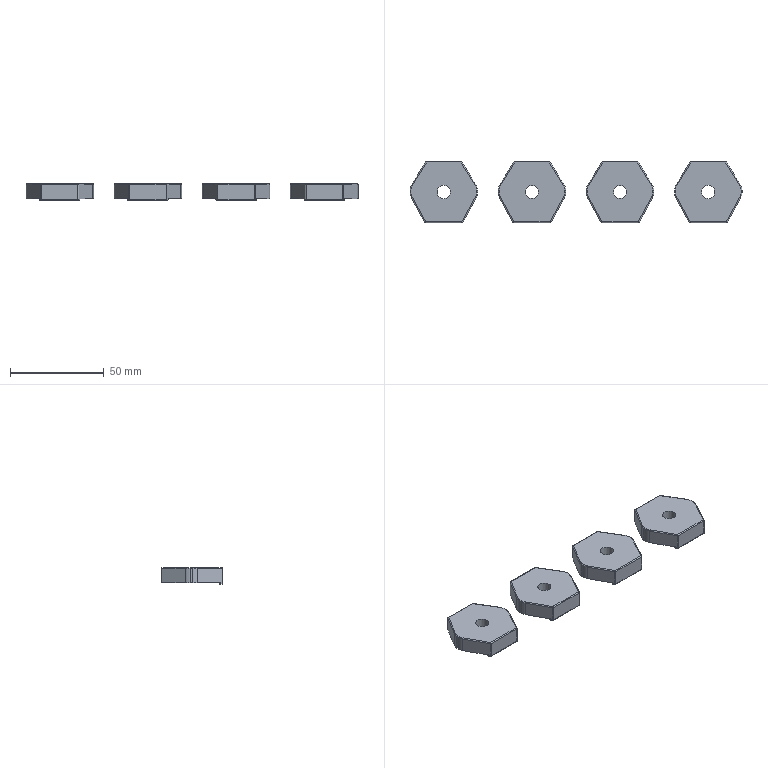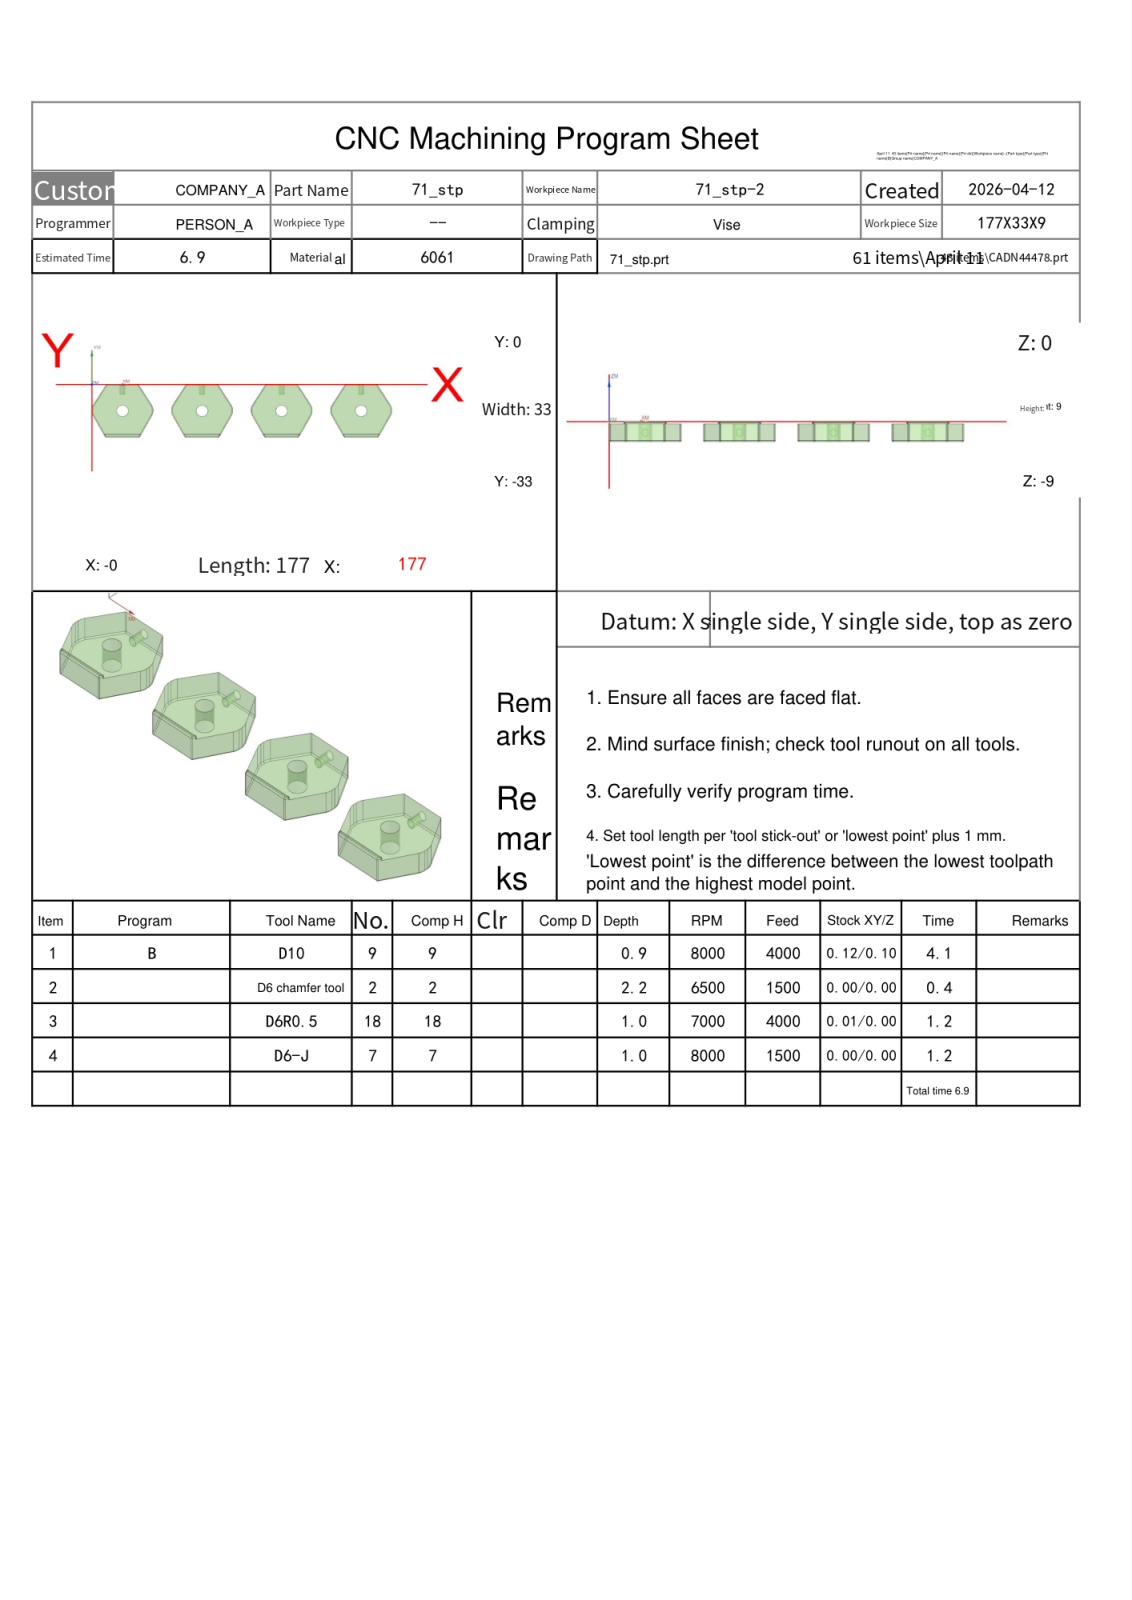NC program | NX | posted by the shop | part box 177 x 33 x 9 mm
Lines 2353 to 3592 of 12693:
N3 T18 M06
(D6R0.5  D=6. R=0.5 H=18 ce=0.01 di=0.00)
G00 G90 G54 X149.909 Y-28.832 M03 S7000
G43 H18 Z50.
M08
Z1.5
G01 X169.408 Z.478 F4000.
X169.836 Y-28.894 Z.455
X170.249 Y-29.023 Z.433
X170.635 Y-29.218 Z.41
X170.985 Y-29.472 Z.387
X171.29 Y-29.78 Z.365
X171.54 Y-30.133 Z.342
X171.731 Y-30.521 Z.319
X171.856 Y-30.935 Z.297
X171.913 Y-31.364 Z.274
X171.9 Y-31.797 Z.251
X171.817 Y-32.221 Z.229
X171.667 Y-32.627 Z.206
X170.97 Y-33.915 Z.129
X170.718 Y-34.255 Z.107
X170.415 Y-34.551 Z.085
X170.07 Y-34.796 Z.063
X169.69 Y-34.983 Z.04
X169.285 Y-35.108 Z.018
X168.866 Y-35.168 Z-.004
X168.702 Z-.012
X149.298
G02 X146.952 Y-33.771 I0.0 J2.668
G01 X146.411 Y-32.771
G02 X146.088 Y-31.5 I2.345 J1.271
X148.756 Y-28.832 I2.668 J0.0
G01 X169.244
G02 X171.912 Y-31.5 I0.0 J-2.668
X171.589 Y-32.771 I-2.668 J0.0
G01 X171.048 Y-33.771
G02 X168.702 Y-35.168 I-2.345 J1.271
G01 X166.277 Y-35.173 Z-.013
X163.851 Y-35.178 Z-.014
X161.426 Y-35.183 Z-.015
X159. Y-35.188 Z-.016
X156.574 Y-35.193 Z-.017
X154.149 Y-35.197 Z-.018
X151.723 Y-35.203 Z-.019
X149.298 Y-35.207 Z-.02
X149.217 Y-35.206
X149.136 Y-35.202
X149.056 Y-35.197
X148.975 Y-35.188
X148.895 Y-35.178
X148.816 Y-35.165
X148.736 Y-35.149
X148.657 Y-35.131
X148.579 Y-35.111
X148.502 Y-35.089
X148.425 Y-35.064
X148.349 Y-35.037
X148.273 Y-35.008
X148.199 Y-34.976
X148.125 Y-34.942
X148.053 Y-34.906
X147.981 Y-34.868
X147.911 Y-34.828
X147.842 Y-34.786
X147.775 Y-34.741
X147.644 Y-34.647
X147.518 Y-34.544
X147.399 Y-34.435
X147.287 Y-34.318 Z-.021
X147.182 Y-34.196
X147.084 Y-34.067
X146.995 Y-33.932
X146.913 Y-33.792
X146.641 Y-33.293
X146.369 Y-32.793
X146.331 Y-32.72
X146.295 Y-32.646
X146.261 Y-32.571
X146.23 Y-32.494
X146.2 Y-32.417
X146.174 Y-32.339
X146.149 Y-32.26
X146.127 Y-32.181
X146.107 Y-32.1
X146.09 Y-32.02
X146.075 Y-31.938 Z-.022
X146.063 Y-31.857
X146.053 Y-31.775
X146.046 Y-31.693
X146.041 Y-31.61
X146.039 Y-31.528
Y-31.445
X146.042 Y-31.362
X146.047 Y-31.28
X146.055 Y-31.198
X146.066 Y-31.116
X146.078 Y-31.034
X146.094 Y-30.953
X146.111 Y-30.872
X146.132 Y-30.792
X146.154 Y-30.713
X146.179 Y-30.634
X146.206 Y-30.556
X146.236 Y-30.479
X146.268 Y-30.402
X146.303 Y-30.327
X146.339 Y-30.253
X146.378 Y-30.18
X146.419 Y-30.109
X146.463 Y-30.038
X146.508 Y-29.969
X146.555 Y-29.901
X146.605 Y-29.835
X146.656 Y-29.77
X146.71 Y-29.707
X146.765 Y-29.646
X146.822 Y-29.586
X146.881 Y-29.528
X146.942 Y-29.472 Z-.023
X147.004 Y-29.418
X147.069 Y-29.365
X147.134 Y-29.315
X147.201 Y-29.266
X147.27 Y-29.22
X147.34 Y-29.176
X147.411 Y-29.134
X147.483 Y-29.094
X147.557 Y-29.056
X147.632 Y-29.021
X147.708 Y-28.987
X147.785 Y-28.957
X147.862 Y-28.928
X147.941 Y-28.902
X148.02 Y-28.878
X148.1 Y-28.857
X148.181 Y-28.838
X148.262 Y-28.822
X148.343 Y-28.808
X148.426 Y-28.797
X148.508 Y-28.787
X148.59 Y-28.781
X148.673 Y-28.777
X148.756 Y-28.776
X151.317 Y-28.772 Z-.024
X153.878 Y-28.768 Z-.025
X156.439 Y-28.763 Z-.026
X159. Y-28.76 Z-.027
X161.561 Y-28.755 Z-.028
X164.122 Y-28.752 Z-.029
X166.683 Y-28.747 Z-.03
X169.244 Y-28.744 Z-.031
X169.328 Y-28.745
X169.412 Y-28.748
X169.495 Y-28.755
X169.579 Y-28.763
X169.662 Y-28.775
X169.744 Y-28.789
X169.826 Y-28.805
X169.908 Y-28.824
X169.989 Y-28.845
X170.07 Y-28.869
X170.149 Y-28.895
X170.228 Y-28.924
X170.306 Y-28.955
X170.383 Y-28.988
X170.459 Y-29.024
X170.534 Y-29.062
X170.607 Y-29.102
X170.679 Y-29.144
X170.751 Y-29.189
X170.82 Y-29.236
X170.888 Y-29.285 Z-.032
X170.955 Y-29.335
X171.02 Y-29.388
X171.083 Y-29.443
X171.145 Y-29.5
X171.205 Y-29.559
X171.263 Y-29.619
X171.32 Y-29.681
X171.374 Y-29.745
X171.427 Y-29.811
X171.477 Y-29.878
X171.525 Y-29.946
X171.572 Y-30.016
X171.616 Y-30.088
X171.658 Y-30.16
X171.697 Y-30.234
X171.735 Y-30.309
X171.77 Y-30.386
X171.803 Y-30.463
X171.833 Y-30.541
X171.862 Y-30.62
X171.887 Y-30.7
X171.91 Y-30.781
X171.931 Y-30.862
X171.949 Y-30.944
X171.965 Y-31.027
X171.978 Y-31.109
X171.989 Y-31.193
X171.997 Y-31.276
X172.003 Y-31.36
X172.006 Y-31.444
Y-31.528
X172.005 Y-31.612 Z-.033
X172. Y-31.696
X171.993 Y-31.78
X171.983 Y-31.863
X171.971 Y-31.946
X171.956 Y-32.029
X171.939 Y-32.111
X171.919 Y-32.193
X171.897 Y-32.274
X171.872 Y-32.354
X171.846 Y-32.434
X171.816 Y-32.512
X171.784 Y-32.59
X171.75 Y-32.667
X171.714 Y-32.743
X171.674 Y-32.817
X171.404 Y-33.317
X171.134 Y-33.818
X171.094 Y-33.89
X171.051 Y-33.961
X171.007 Y-34.03
X170.96 Y-34.098 Z-.034
X170.912 Y-34.165
X170.861 Y-34.23
X170.809 Y-34.294
X170.754 Y-34.356
X170.698 Y-34.417
X170.64 Y-34.475
X170.58 Y-34.532
X170.519 Y-34.587
X170.456 Y-34.641
X170.391 Y-34.692
X170.325 Y-34.742
X170.258 Y-34.789
X170.189 Y-34.835
X170.118 Y-34.878
X170.047 Y-34.92
X169.974 Y-34.958
X169.9 Y-34.996
X169.825 Y-35.03
X169.75 Y-35.063
X169.672 Y-35.093
X169.595 Y-35.121
X169.516 Y-35.147
X169.437 Y-35.17
X169.357 Y-35.19
X169.276 Y-35.209
X169.195 Y-35.225
X169.114 Y-35.239
X169.032 Y-35.25
X168.867 Y-35.265
X168.702 Y-35.27 Z-.035
X166.277 Y-35.275 Z-.036
X163.851 Y-35.28 Z-.037
X161.426 Y-35.284 Z-.038
X159. Y-35.288 Z-.04
X156.574 Y-35.293 Z-.041
X154.149 Y-35.297 Z-.042
X151.723 Y-35.301 Z-.043
X149.298 Y-35.305 Z-.045
X149.214
X149.13 Y-35.301
X149.047 Y-35.295
X148.964 Y-35.286
X148.881 Y-35.275
X148.798 Y-35.261
X148.716 Y-35.246
X148.634 Y-35.227
X148.553 Y-35.206
X148.473 Y-35.183
X148.393 Y-35.157
X148.314 Y-35.129
X148.236 Y-35.099
X148.159 Y-35.066
X148.083 Y-35.031
X148.008 Y-34.994
X147.934 Y-34.955 Z-.046
X147.861 Y-34.913
X147.789 Y-34.869
X147.72 Y-34.823
X147.651 Y-34.775
X147.584 Y-34.725
X147.518 Y-34.673
X147.454 Y-34.619
X147.391 Y-34.563
X147.331 Y-34.505
X147.271 Y-34.446
X147.214 Y-34.385
X147.159 Y-34.322
X147.105 Y-34.257
X147.053 Y-34.191
X147.004 Y-34.123
X146.956 Y-34.054
X146.911 Y-33.984
X146.868 Y-33.912
X146.827 Y-33.839
X146.555 Y-33.339 Z-.047
X146.283 Y-32.84
X146.21 Y-32.696
X146.145 Y-32.548
X146.089 Y-32.396
X146.042 Y-32.242
X146.004 Y-32.085
X145.974 Y-31.926
X145.954 Y-31.766 Z-.048
X145.943 Y-31.605
X145.942 Y-31.443
X145.949 Y-31.281
X145.966 Y-31.121
X145.992 Y-30.961
X146.027 Y-30.803
X146.072 Y-30.648
X146.125 Y-30.495
X146.186 Y-30.346
X146.257 Y-30.2
X146.335 Y-30.058 Z-.049
X146.422 Y-29.922
X146.516 Y-29.79
X146.618 Y-29.664
X146.726 Y-29.544
X146.842 Y-29.431
X146.963 Y-29.324
X147.091 Y-29.225
X147.224 Y-29.133
X147.363 Y-29.049
X147.505 Y-28.972
X147.652 Y-28.905
X147.803 Y-28.845 Z-.05
X147.957 Y-28.795
X148.114 Y-28.753
X148.272 Y-28.72
X148.433 Y-28.697
X148.594 Y-28.683
X148.756 Y-28.678
X151.317 Y-28.674 Z-.051
X153.878 Y-28.67 Z-.053
X156.439 Y-28.666 Z-.054
X159. Y-28.662 Z-.055
X161.561 Y-28.658 Z-.057
X164.122 Y-28.654 Z-.058
X166.683 Y-28.65 Z-.06
X169.244 Y-28.647 Z-.061
X169.408 Y-28.651
X169.571 Y-28.665
X169.733 Y-28.688
X169.894 Y-28.721
X170.053 Y-28.762
X170.208 Y-28.813
X170.361 Y-28.873
X170.51 Y-28.941 Z-.062
X170.655 Y-29.018
X170.796 Y-29.102
X170.931 Y-29.195
X171.06 Y-29.295
X171.184 Y-29.403
X171.301 Y-29.518
X171.412 Y-29.639
X171.515 Y-29.766
X171.611 Y-29.9
X171.699 Y-30.038
X171.779 Y-30.181 Z-.063
X171.851 Y-30.329
X171.914 Y-30.48
X171.969 Y-30.635
X172.014 Y-30.793
X172.05 Y-30.953
X172.077 Y-31.115
X172.095 Y-31.278
X172.103 Y-31.442
X172.102 Y-31.606
X172.091 Y-31.77
X172.071 Y-31.933
X172.042 Y-32.095 Z-.064
X172.004 Y-32.254
X171.956 Y-32.412
X171.899 Y-32.566
X171.834 Y-32.717
X171.76 Y-32.863
X171.49 Y-33.364
X171.22 Y-33.864 Z-.065
X171.178 Y-33.939
X171.134 Y-34.012
X171.088 Y-34.084
X171.04 Y-34.154
X170.99 Y-34.224
X170.937 Y-34.291
X170.883 Y-34.357
X170.826 Y-34.421
X170.768 Y-34.484
X170.708 Y-34.545
X170.647 Y-34.604
X170.583 Y-34.661
X170.518 Y-34.716
X170.451 Y-34.769
X170.382 Y-34.821
X170.312 Y-34.87
X170.241 Y-34.917
X170.168 Y-34.962
X170.094 Y-35.005
X170.019 Y-35.045 Z-.066
X169.943 Y-35.084
X169.865 Y-35.119
X169.786 Y-35.153
X169.707 Y-35.184
X169.626 Y-35.213
X169.545 Y-35.24
X169.463 Y-35.264
X169.38 Y-35.285
X169.297 Y-35.305
X169.213 Y-35.321
X169.128 Y-35.335
X169.044 Y-35.347
X168.959 Y-35.356
X168.873 Y-35.362
X168.788 Y-35.366
X168.702 Y-35.368
X166.277 Y-35.372 Z-.068
X163.851 Y-35.376 Z-.07
X161.426 Y-35.38 Z-.071
X159. Y-35.384 Z-.073
X156.574 Y-35.388 Z-.074
X154.149 Y-35.392 Z-.076
X151.723 Y-35.396 Z-.078
X149.298 Y-35.4 Z-.079
X149.142 Y-35.396
X148.987 Y-35.384 Z-.08
X148.832 Y-35.363
X148.679 Y-35.334
X148.528 Y-35.297
X148.379 Y-35.252
X148.232 Y-35.199
X148.089 Y-35.138
X147.949 Y-35.07
X147.813 Y-34.994
X147.681 Y-34.911 Z-.081
X147.554 Y-34.821
X147.431 Y-34.724
X147.314 Y-34.621
X147.203 Y-34.511
X147.098 Y-34.396
X146.999 Y-34.275
X146.907 Y-34.15
X146.822 Y-34.019
X146.744 Y-33.884
X146.472 Y-33.384 Z-.082
X146.2 Y-32.885
X146.125 Y-32.736
X146.058 Y-32.583
X146. Y-32.426 Z-.083
X145.951 Y-32.267
X145.911 Y-32.105
X145.881 Y-31.94
X145.86 Y-31.775
X145.849 Y-31.608
X145.847 Y-31.441
X145.855 Y-31.274
X145.873 Y-31.108
X145.9 Y-30.943 Z-.084
X145.936 Y-30.78
X145.982 Y-30.619
X146.037 Y-30.461
X146.1 Y-30.307
X146.173 Y-30.156
X146.254 Y-30.01
X146.344 Y-29.869
X146.441 Y-29.733 Z-.085
X146.546 Y-29.603
X146.658 Y-29.479
X146.778 Y-29.362
X146.903 Y-29.251
X147.036 Y-29.149
X147.173 Y-29.054
X147.316 Y-28.967
X147.464 Y-28.888
X147.616 Y-28.818 Z-.086
X147.771 Y-28.756
X147.93 Y-28.704
X148.092 Y-28.661
X148.256 Y-28.628
X148.422 Y-28.603
X148.589 Y-28.589
X148.756 Y-28.584
X151.317 Y-28.58 Z-.088
X153.878 Y-28.576 Z-.09
X156.439 Y-28.573 Z-.092
X159. Y-28.569 Z-.093
X161.561 Y-28.565 Z-.095
X164.122 Y-28.561 Z-.097
X166.683 Y-28.558 Z-.098
X169.244 Y-28.554 Z-.1
X169.413 Y-28.559
X169.582 Y-28.573
X169.749 Y-28.597 Z-.101
X169.915 Y-28.63
X170.079 Y-28.673
X170.24 Y-28.726
X170.397 Y-28.787
X170.551 Y-28.858
X170.701 Y-28.937
X170.846 Y-29.024
X170.985 Y-29.12
X171.119 Y-29.224 Z-.102
X171.247 Y-29.335
X171.368 Y-29.453
X171.482 Y-29.579
X171.589 Y-29.71
X171.688 Y-29.848
X171.779 Y-29.99
X171.862 Y-30.138
X171.936 Y-30.291
X172.001 Y-30.447 Z-.103
X172.057 Y-30.607
X172.104 Y-30.77
X172.141 Y-30.935
X172.169 Y-31.102
X172.188 Y-31.271
X172.196 Y-31.44
X172.195 Y-31.61
X172.184 Y-31.779 Z-.104
X172.163 Y-31.947
X172.133 Y-32.114
X172.093 Y-32.279
X172.044 Y-32.441
X171.986 Y-32.6
X171.918 Y-32.756
X171.842 Y-32.908
X171.571 Y-33.408 Z-.105
X171.301 Y-33.908
X171.222 Y-34.046
X171.136 Y-34.179
X171.042 Y-34.307
X170.942 Y-34.431 Z-.106
X170.835 Y-34.548
X170.722 Y-34.66
X170.604 Y-34.765
X170.479 Y-34.864
X170.35 Y-34.957
X170.216 Y-35.042
X170.077 Y-35.119
X169.935 Y-35.19
X169.789 Y-35.252
X169.639 Y-35.307 Z-.107
X169.487 Y-35.353
X169.333 Y-35.391
X169.177 Y-35.421
X169.02 Y-35.443
X168.861 Y-35.456
X168.702 Y-35.461
X166.277 Y-35.464 Z-.109
X163.851 Y-35.468 Z-.111
X161.426 Y-35.472 Z-.113
X159. Y-35.476 Z-.115
X156.574 Y-35.48 Z-.117
X154.149 Y-35.483 Z-.119
X151.723 Y-35.487 Z-.121
X149.298 Y-35.49 Z-.123
X149.137 Y-35.486
X148.977 Y-35.473
X148.818 Y-35.452
X148.66 Y-35.422 Z-.124
X148.504 Y-35.384
X148.35 Y-35.338
X148.199 Y-35.283
X148.051 Y-35.22
X147.907 Y-35.15
X147.767 Y-35.071
X147.63 Y-34.986 Z-.125
X147.499 Y-34.893
X147.373 Y-34.793
X147.253 Y-34.686
X147.138 Y-34.574
X147.03 Y-34.455
X146.928 Y-34.331
X146.833 Y-34.201
X146.745 Y-34.066 Z-.126
X146.664 Y-33.927
X146.393 Y-33.427
X146.121 Y-32.928 Z-.127
X146.081 Y-32.852
X146.043 Y-32.774
X146.007 Y-32.696
X145.974 Y-32.617
X145.943 Y-32.536
X145.915 Y-32.455
X145.888 Y-32.373
X145.864 Y-32.291
X145.842 Y-32.207
X145.823 Y-32.123
X145.806 Y-32.039
X145.792 Y-31.954
X145.78 Y-31.869 Z-.128
X145.771 Y-31.783
X145.764 Y-31.697
X145.759 Y-31.611
X145.757 Y-31.525
Y-31.439
X145.76 Y-31.353
X145.766 Y-31.267
X145.773 Y-31.181
X145.784 Y-31.096
X145.796 Y-31.011
X145.811 Y-30.926
X145.829 Y-30.842
X145.849 Y-30.758
X145.871 Y-30.675 Z-.129
X145.896 Y-30.592
X145.923 Y-30.51
X145.953 Y-30.429
X145.984 Y-30.349
X146.019 Y-30.27
X146.055 Y-30.192
X146.093 Y-30.115
X146.134 Y-30.039
X146.177 Y-29.964
X146.222 Y-29.891
X146.269 Y-29.819
X146.318 Y-29.748
X146.37 Y-29.679
X146.423 Y-29.611 Z-.13
X146.478 Y-29.544
X146.535 Y-29.48
X146.594 Y-29.417
X146.654 Y-29.355
X146.717 Y-29.296
X146.781 Y-29.238
X146.846 Y-29.182
X146.914 Y-29.128
X146.982 Y-29.076
X147.053 Y-29.026
X147.124 Y-28.978
X147.197 Y-28.932
X147.272 Y-28.889
X147.347 Y-28.847 Z-.131
X147.424 Y-28.807
X147.502 Y-28.77
X147.58 Y-28.735
X147.66 Y-28.703
X147.741 Y-28.672
X147.823 Y-28.644
X147.905 Y-28.618
X147.988 Y-28.595
X148.072 Y-28.574
X148.156 Y-28.555
X148.241 Y-28.539
X148.326 Y-28.526
X148.411 Y-28.514
X148.497 Y-28.506
X148.583 Y-28.499 Z-.132
X148.67 Y-28.495
X148.756 Y-28.494
X151.317 Y-28.491 Z-.134
X153.878 Y-28.487 Z-.136
X156.439 Y-28.484 Z-.138
X159. Y-28.48 Z-.14
X161.561 Y-28.477 Z-.142
X164.122 Y-28.473 Z-.144
X166.683 Y-28.469 Z-.146
X169.244 Y-28.466 Z-.148
X169.331 Y-28.467 Z-.149
X169.418 Y-28.471
X169.505 Y-28.477
X169.592 Y-28.486
X169.678 Y-28.496
X169.764 Y-28.51
X169.85 Y-28.526
X169.935 Y-28.545
X170.02 Y-28.566
X170.104 Y-28.589
X170.187 Y-28.615
X170.269 Y-28.643
X170.351 Y-28.673
X170.432 Y-28.706
X170.512 Y-28.741
X170.59 Y-28.779 Z-.15
X170.668 Y-28.818
X170.744 Y-28.86
X170.82 Y-28.904
X170.894 Y-28.951
X170.966 Y-28.999
X171.037 Y-29.049
X171.107 Y-29.102
X171.175 Y-29.156
X171.242 Y-29.212
X171.307 Y-29.271
X171.37 Y-29.331
X171.431 Y-29.393
X171.491 Y-29.456
X171.549 Y-29.521 Z-.151
X171.605 Y-29.588
X171.659 Y-29.657
X171.711 Y-29.727
X171.761 Y-29.798
X171.809 Y-29.871
X171.855 Y-29.945
X171.898 Y-30.021
X171.94 Y-30.098
X171.979 Y-30.176
X172.016 Y-30.255
X172.051 Y-30.335
X172.083 Y-30.416
X172.113 Y-30.498
X172.141 Y-30.58 Z-.152
X172.166 Y-30.664
X172.189 Y-30.748
X172.21 Y-30.833
X172.228 Y-30.918
X172.243 Y-31.004
X172.256 Y-31.09
X172.267 Y-31.177
X172.275 Y-31.264
X172.281 Y-31.351
X172.284 Y-31.438
Y-31.526
X172.283 Y-31.613
X172.278 Y-31.7
X172.271 Y-31.787 Z-.153
X172.262 Y-31.874
X172.25 Y-31.96
X172.236 Y-32.047
X172.219 Y-32.132
X172.2 Y-32.217
X172.178 Y-32.302
X172.154 Y-32.386
X172.127 Y-32.469
X172.098 Y-32.552
X172.067 Y-32.633
X172.034 Y-32.714
X171.998 Y-32.793
X171.959 Y-32.872
X171.919 Y-32.949 Z-.154
X171.649 Y-33.45
X171.378 Y-33.95
X171.297 Y-34.092 Z-.155
X171.208 Y-34.229
X171.112 Y-34.361
X171.008 Y-34.488
X170.898 Y-34.609
X170.782 Y-34.724
X170.66 Y-34.833
X170.532 Y-34.934 Z-.156
X170.399 Y-35.029
X170.261 Y-35.117
X170.118 Y-35.197
X169.971 Y-35.269
X169.821 Y-35.334
X169.667 Y-35.39
X169.511 Y-35.438
X169.352 Y-35.477 Z-.157
X169.191 Y-35.508
X169.029 Y-35.53
X168.866 Y-35.543
X168.702 Y-35.548
X166.277 Y-35.551 Z-.159
X163.851 Y-35.555 Z-.162
X161.426 Y-35.558 Z-.164
X159. Y-35.562 Z-.166
X156.574 Y-35.566 Z-.169
X154.149 Y-35.569 Z-.171
X151.723 Y-35.573 Z-.173
X149.298 Y-35.575 Z-.176
X149.133 Y-35.571
X148.968 Y-35.558
X148.804 Y-35.536
X148.642 Y-35.506
X148.481 Y-35.466
X148.323 Y-35.418
X148.168 Y-35.362 Z-.177
X148.016 Y-35.298
X147.867 Y-35.225
X147.723 Y-35.144
X147.583 Y-35.056
X147.448 Y-34.961
X147.319 Y-34.858 Z-.178
X147.195 Y-34.749
X147.077 Y-34.633
X146.965 Y-34.51
X146.861 Y-34.382
X146.763 Y-34.249
X146.672 Y-34.111
X146.59 Y-33.967 Z-.179
X146.318 Y-33.468
X146.046 Y-32.968 Z-.18
X145.97 Y-32.819
X145.903 Y-32.665
X145.843 Y-32.509
X145.792 Y-32.349
X145.75 Y-32.186 Z-.181
X145.717 Y-32.022
X145.693 Y-31.856
X145.678 Y-31.689
X145.672 Y-31.521
X145.675 Y-31.354
X145.688 Y-31.186
X145.709 Y-31.02 Z-.182
X145.739 Y-30.855
X145.779 Y-30.692
X145.827 Y-30.531
X145.884 Y-30.373
X145.949 Y-30.218
X146.023 Y-30.068 Z-.183
X146.104 Y-29.921
X146.194 Y-29.779
X146.291 Y-29.642
X146.396 Y-29.511
X146.507 Y-29.385
X146.625 Y-29.266 Z-.184
X146.75 Y-29.153
X146.88 Y-29.047
X147.016 Y-28.949
X147.157 Y-28.858
X147.303 Y-28.775
X147.454 Y-28.699
X147.608 Y-28.633 Z-.185
X147.765 Y-28.574
X147.926 Y-28.524
X148.089 Y-28.483
X148.254 Y-28.451
X148.42 Y-28.428
X148.588 Y-28.415 Z-.186
X148.756 Y-28.41
X151.317 Y-28.406 Z-.188
X153.878 Y-28.403 Z-.191
X156.439 Y-28.4 Z-.193
X159. Y-28.397 Z-.195
X161.561 Y-28.393 Z-.198
X164.122 Y-28.39 Z-.2
X166.683 Y-28.387 Z-.203
X169.244 Y-28.383 Z-.205
X169.414 Y-28.388
X169.583 Y-28.402
X169.751 Y-28.424 Z-.206
X169.917 Y-28.456
X170.082 Y-28.497
X170.244 Y-28.547
X170.403 Y-28.605
X170.559 Y-28.673
X170.711 Y-28.748 Z-.207
X170.858 Y-28.832
X171.001 Y-28.923
X171.139 Y-29.022
X171.271 Y-29.129
X171.397 Y-29.242
X171.517 Y-29.363 Z-.208
X171.63 Y-29.489
X171.736 Y-29.622
X171.834 Y-29.76
X171.925 Y-29.903
X172.008 Y-30.051
X172.083 Y-30.204
X172.15 Y-30.36 Z-.209
X172.207 Y-30.52
X172.257 Y-30.682
X172.297 Y-30.847
X172.328 Y-31.014
X172.35 Y-31.182
X172.363 Y-31.352 Z-.21
X172.367 Y-31.522
X172.361 Y-31.691
X172.346 Y-31.861
X172.322 Y-32.029
X172.289 Y-32.195
X172.247 Y-32.36 Z-.211
X172.196 Y-32.522
X172.136 Y-32.681
X172.068 Y-32.837
X171.991 Y-32.989
X171.721 Y-33.489 Z-.212
X171.45 Y-33.989
X171.367 Y-34.135
X171.275 Y-34.276 Z-.213
X171.176 Y-34.411
X171.071 Y-34.541
X170.958 Y-34.666
X170.838 Y-34.784
X170.713 Y-34.895
X170.581 Y-35. Z-.214
X170.444 Y-35.097
X170.303 Y-35.187
X170.156 Y-35.27
X170.005 Y-35.344
X169.851 Y-35.41
X169.693 Y-35.468 Z-.215
X169.532 Y-35.517
X169.369 Y-35.557
X169.204 Y-35.589
X169.038 Y-35.611
X168.87 Y-35.625
X168.702 Y-35.63
X166.277 Y-35.633 Z-.218
X163.851 Y-35.636 Z-.221
X161.426 Y-35.64 Z-.223
X159. Y-35.643 Z-.226
X156.574 Y-35.646 Z-.228
X154.149 Y-35.649 Z-.231
X151.723 Y-35.652 Z-.234
X149.298 Y-35.655 Z-.236
X149.128 Y-35.651
X148.959 Y-35.637
X148.791 Y-35.615 Z-.237
X148.625 Y-35.583
X148.46 Y-35.543
X148.298 Y-35.494
X148.139 Y-35.436
X147.983 Y-35.37 Z-.238
X147.83 Y-35.295
X147.682 Y-35.213
X147.539 Y-35.122
X147.401 Y-35.024
X147.268 Y-34.919
X147.141 Y-34.806 Z-.239
X147.02 Y-34.688
X146.905 Y-34.562
X146.798 Y-34.431
X146.698 Y-34.294
X146.605 Y-34.152 Z-.24
X146.52 Y-34.005
X146.248 Y-33.506
X145.977 Y-33.006 Z-.241
X145.899 Y-32.853
X145.829 Y-32.695
X145.769 Y-32.534
X145.716 Y-32.371 Z-.242
X145.673 Y-32.204
X145.639 Y-32.035
X145.615 Y-31.865
X145.599 Y-31.694
X145.593 Y-31.522 Z-.243
X145.597 Y-31.35
X145.609 Y-31.178
X145.631 Y-31.008
X145.662 Y-30.838
X145.703 Y-30.671
X145.752 Y-30.506 Z-.244
X145.81 Y-30.344
X145.877 Y-30.186
X145.953 Y-30.031
X146.037 Y-29.881
X146.129 Y-29.735 Z-.245
X146.228 Y-29.595
X146.335 Y-29.46
X146.45 Y-29.331
X146.571 Y-29.209
X146.699 Y-29.093 Z-.246
X146.832 Y-28.985
X146.972 Y-28.884
X147.117 Y-28.79
X147.266 Y-28.705
X147.42 Y-28.628
X147.579 Y-28.56 Z-.247
X147.74 Y-28.5
X147.905 Y-28.449
X148.072 Y-28.407
X148.241 Y-28.374
X148.412 Y-28.35 Z-.248
X148.584 Y-28.336
X148.756 Y-28.331
X151.317 Y-28.329 Z-.251
X153.878 Y-28.325 Z-.253
X156.439 Y-28.322 Z-.256
X159. Y-28.319 Z-.259
X161.561 Y-28.316 Z-.262
X164.122 Y-28.313 Z-.264
X166.683 Y-28.31 Z-.267
X169.244 Y-28.307 Z-.27
X169.418 Y-28.312
X169.591 Y-28.326
X169.763 Y-28.349
X169.934 Y-28.382
X170.102 Y-28.424 Z-.271
X170.268 Y-28.475
X170.431 Y-28.535
X170.591 Y-28.603
X170.747 Y-28.681
X170.898 Y-28.766 Z-.272
X171.044 Y-28.86
X171.185 Y-28.962
X171.32 Y-29.071
X171.449 Y-29.187
X171.572 Y-29.311
X171.688 Y-29.44 Z-.273
X171.796 Y-29.576
X171.897 Y-29.718
X171.991 Y-29.864
X172.076 Y-30.016
X172.152 Y-30.172 Z-.274
X172.22 Y-30.332
X172.28 Y-30.496
X172.33 Y-30.662
X172.371 Y-30.831
X172.403 Y-31.002
X172.426 Y-31.175 Z-.275
X172.439 Y-31.348
X172.443 Y-31.522
X172.437 Y-31.696
X172.422 Y-31.869
X172.397 Y-32.042 Z-.276
X172.363 Y-32.212
X172.32 Y-32.381
X172.268 Y-32.547
X172.207 Y-32.71
X172.136 Y-32.869 Z-.277
X172.058 Y-33.025
X171.788 Y-33.525
X171.517 Y-34.025 Z-.278
X171.431 Y-34.174
X171.338 Y-34.319
X171.236 Y-34.457
X171.128 Y-34.591 Z-.279
X171.012 Y-34.718
X170.89 Y-34.839
X170.761 Y-34.953
X170.627 Y-35.061
X170.487 Y-35.16 Z-.28
X170.341 Y-35.253
X170.191 Y-35.337
X170.037 Y-35.413
X169.879 Y-35.48
X169.717 Y-35.539
X169.552 Y-35.59 Z-.281
X169.385 Y-35.631
X169.216 Y-35.663
X169.046 Y-35.687
X168.874 Y-35.701
X168.702 Y-35.706 Z-.282
X166.277 Y-35.708 Z-.284
X163.851 Y-35.711 Z-.287
X161.426 Y-35.714 Z-.29
X159. Y-35.717 Z-.293
X156.574 Y-35.72 Z-.296
X154.149 Y-35.722 Z-.299
X151.723 Y-35.725 Z-.301
X149.298 Y-35.728 Z-.304
X149.124 Y-35.724 Z-.305
X148.952 Y-35.71
X148.78 Y-35.687
X148.609 Y-35.655
X148.441 Y-35.613
X148.275 Y-35.563 Z-.306
X148.112 Y-35.504
X147.952 Y-35.436
X147.797 Y-35.36
X147.645 Y-35.275
X147.498 Y-35.183 Z-.307
X147.357 Y-35.082
X147.221 Y-34.975
X147.091 Y-34.86
X146.967 Y-34.738
X146.85 Y-34.61 Z-.308
X146.74 Y-34.475
X146.638 Y-34.335
X146.543 Y-34.19
X146.456 Y-34.04
X146.185 Y-33.54 Z-.309
X145.913 Y-33.04 Z-.31
X145.833 Y-32.884
X145.762 Y-32.723
X145.7 Y-32.558
X145.647 Y-32.391 Z-.311
X145.603 Y-32.22
X145.568 Y-32.048
X145.543 Y-31.874
X145.527 Y-31.698
X145.521 Y-31.522 Z-.312
X145.524 Y-31.346
X145.537 Y-31.171
X145.559 Y-30.996
X145.592 Y-30.823
X145.633 Y-30.652 Z-.313
X145.684 Y-30.484
X145.743 Y-30.318
X145.812 Y-30.156
X145.889 Y-29.997
X145.975 Y-29.844 Z-.314
X146.069 Y-29.695
X146.171 Y-29.551
X146.28 Y-29.413
X146.397 Y-29.282
X146.521 Y-29.157 Z-.315
X146.652 Y-29.039
X146.789 Y-28.928
X146.931 Y-28.824
X147.079 Y-28.729
X147.233 Y-28.642 Z-.316
X147.39 Y-28.563
X147.552 Y-28.493
X147.717 Y-28.432
X147.885 Y-28.379 Z-.317
X148.056 Y-28.336
X148.229 Y-28.303
X148.404 Y-28.279
X148.58 Y-28.264
X148.756 Y-28.259 Z-.318
X151.317 Y-28.256 Z-.321
X153.878 Y-28.254 Z-.324
X156.439 Y-28.251 Z-.327
X159. Y-28.249 Z-.33
X161.561 Y-28.246 Z-.333
X164.122 Y-28.243 Z-.336
X166.683 Y-28.241 Z-.339
X169.244 Y-28.238 Z-.342
X169.422 Y-28.242
X169.598 Y-28.257
X169.774 Y-28.281
X169.949 Y-28.314
X170.121 Y-28.357 Z-.343
X170.291 Y-28.409
X170.457 Y-28.47
X170.62 Y-28.54
X170.779 Y-28.62
X170.934 Y-28.707 Z-.344
X171.083 Y-28.803
X171.227 Y-28.907
X171.365 Y-29.018
X171.497 Y-29.137
X171.623 Y-29.263 Z-.345
X171.741 Y-29.396
X171.852 Y-29.534
X171.955 Y-29.679
X172.05 Y-29.829
X172.137 Y-29.984 Z-.346
X172.215 Y-30.144
X172.285 Y-30.307
X172.345 Y-30.474
X172.397 Y-30.644 Z-.347
X172.439 Y-30.817
X172.471 Y-30.991
X172.494 Y-31.168
X172.508 Y-31.345
X172.512 Y-31.523 Z-.348
X172.506 Y-31.7
X172.49 Y-31.877
X172.465 Y-32.053
X172.43 Y-32.228
X172.386 Y-32.4 Z-.349
X172.333 Y-32.57
X172.27 Y-32.736
X172.199 Y-32.899
X172.119 Y-33.058
X171.848 Y-33.558 Z-.35
X171.578 Y-34.058 Z-.351
X171.49 Y-34.21
X171.394 Y-34.358
X171.291 Y-34.499
X171.18 Y-34.636 Z-.352
X171.062 Y-34.766
X170.937 Y-34.889
X170.805 Y-35.006
X170.668 Y-35.115
X170.525 Y-35.217 Z-.353
X170.376 Y-35.311
X170.223 Y-35.397
X170.066 Y-35.475
X169.904 Y-35.544
X169.739 Y-35.604 Z-.354
X169.571 Y-35.656
X169.4 Y-35.698
X169.227 Y-35.731
X169.053 Y-35.755
X168.878 Y-35.769 Z-.355
X168.702 Y-35.774
X166.277 Y-35.776 Z-.358
X163.851 Y-35.779 Z-.361
X161.426 Y-35.781 Z-.364
X159. Y-35.784 Z-.367
X156.574 Y-35.787 Z-.37
X154.149 Y-35.789 Z-.373
X151.723 Y-35.792 Z-.376
X149.298 Y-35.794 Z-.379
X149.121 Y-35.789 Z-.38
X148.945 Y-35.775
X148.769 Y-35.752
X148.595 Y-35.719
X148.424 Y-35.677 Z-.381
X148.254 Y-35.625
X148.088 Y-35.565
X147.925 Y-35.496
X147.766 Y-35.418
X147.611 Y-35.332 Z-.382
X147.462 Y-35.237
X147.317 Y-35.135
X147.179 Y-35.025
X147.046 Y-34.908 Z-.383
X146.92 Y-34.783
X146.801 Y-34.653
X146.689 Y-34.515
X146.584 Y-34.373
X146.487 Y-34.224 Z-.384
X146.398 Y-34.071
X146.128 Y-33.571 Z-.385
X145.856 Y-33.072
X145.775 Y-32.911 Z-.386
X145.702 Y-32.747
X145.639 Y-32.579
X145.584 Y-32.409
X145.539 Y-32.235
X145.504 Y-32.059 Z-.387
X145.478 Y-31.881
X145.462 Y-31.702
X145.456 Y-31.523
X145.459 Y-31.343 Z-.388
X145.473 Y-31.164
X145.495 Y-30.986
X145.528 Y-30.81
X145.57 Y-30.635 Z-.389
X145.622 Y-30.463
X145.682 Y-30.294
X145.753 Y-30.129
X145.831 Y-29.967
X145.919 Y-29.811 Z-.39
X146.015 Y-29.659
X146.119 Y-29.512
X146.231 Y-29.372
X146.35 Y-29.237 Z-.391
X146.477 Y-29.11
X146.61 Y-28.989
X146.749 Y-28.876
X146.895 Y-28.771
X147.046 Y-28.673 Z-.392
X147.202 Y-28.585
X147.363 Y-28.504
X147.528 Y-28.433
X147.696 Y-28.37 Z-.393
X147.868 Y-28.317
X148.042 Y-28.273
X148.219 Y-28.239
X148.397 Y-28.215 Z-.394
X148.576 Y-28.2
X148.756 Y-28.195
X151.317 Y-28.193 Z-.397
X153.878 Y-28.19 Z-.4
X156.439 Y-28.188 Z-.404
X159. Y-28.185 Z-.407
X161.561 Y-28.183 Z-.41
X164.122 Y-28.18 Z-.413
X166.683 Y-28.179 Z-.417
X169.244 Y-28.176 Z-.42
X169.425 Y-28.181